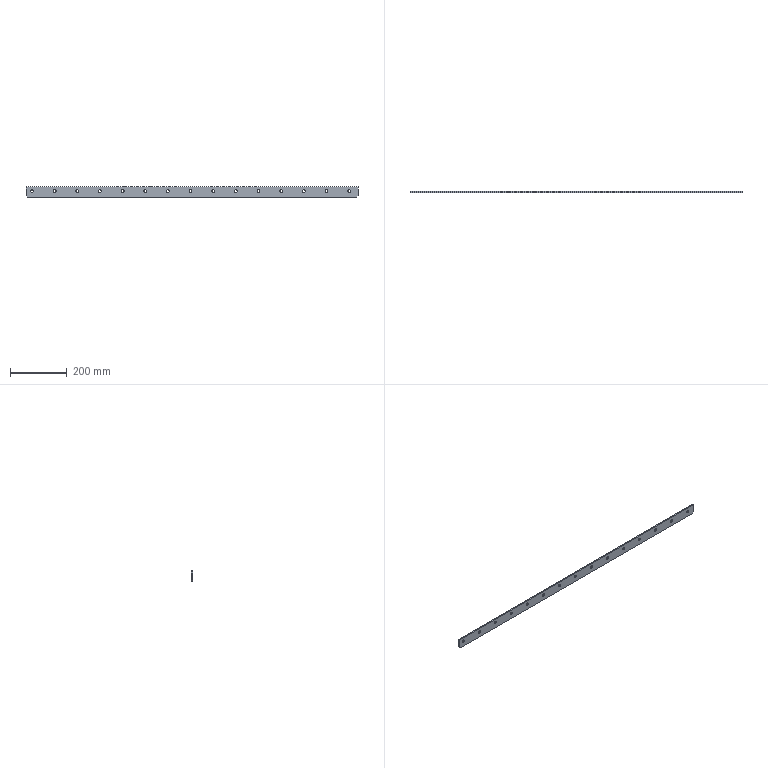Part | SolidWorks | features Chamfer 1, Extrusion 1, HoleWzd 1, LPattern 1 | 1 solid | 38 faces | box 1172 x 4 x 36 mm | volume 163956 mm3 | cylinder 30 | plane 8 | commonest cylinder face diameters 10 x30
STEP:
#1=CARTESIAN_POINT('',(-31.,0.,16.));
#2=VERTEX_POINT('',#1);
#3=CARTESIAN_POINT('',(-31.,0.,26.));
#4=VERTEX_POINT('',#3);
#5=CARTESIAN_POINT('',(-31.,0.,21.));
#6=DIRECTION('',(0.,1.,0.));
#7=DIRECTION('',(0.,0.,1.));
#8=AXIS2_PLACEMENT_3D('',#5,#6,#7);
#9=CIRCLE('',#8,5.);
#10=EDGE_CURVE('',#2,#4,#9,.T.);
#11=ORIENTED_EDGE('',*,*,#10,.F.);
#12=CARTESIAN_POINT('',(-31.,4.,16.));
#13=VERTEX_POINT('',#12);
#14=CARTESIAN_POINT('',(-31.,4.,16.));
#15=DIRECTION('',(0.,1.,0.));
#16=VECTOR('',#15,1000.);
#17=LINE('',#14,#16);
#18=EDGE_CURVE('',#2,#13,#17,.T.);
#19=ORIENTED_EDGE('',*,*,#18,.T.);
#20=CARTESIAN_POINT('',(-31.,4.,26.));
#21=VERTEX_POINT('',#20);
#22=CARTESIAN_POINT('',(-31.,4.,21.));
#23=DIRECTION('',(0.,1.,0.));
#24=DIRECTION('',(0.,0.,1.));
#25=AXIS2_PLACEMENT_3D('',#22,#23,#24);
#26=CIRCLE('',#25,5.);
#27=EDGE_CURVE('',#13,#21,#26,.T.);
#28=ORIENTED_EDGE('',*,*,#27,.T.);
#29=CARTESIAN_POINT('',(-31.,4.,26.));
#30=DIRECTION('',(0.,1.,0.));
#31=VECTOR('',#30,1000.);
#32=LINE('',#29,#31);
#33=EDGE_CURVE('',#4,#21,#32,.T.);
#34=ORIENTED_EDGE('',*,*,#33,.F.);
#35=EDGE_LOOP('',(#11,#19,#28,#34));
#36=FACE_OUTER_BOUND('',#35,.T.);
#37=CARTESIAN_POINT('',(-31.,4.,21.));
#38=DIRECTION('',(0.,1.,0.));
#39=DIRECTION('',(0.,0.,1.));
#40=AXIS2_PLACEMENT_3D('',#37,#38,#39);
#41=CYLINDRICAL_SURFACE('',#40,5.);
#42=ADVANCED_FACE('',(#36),#41,.F.);
#43=CARTESIAN_POINT('',(-111.,0.,16.));
#44=VERTEX_POINT('',#43);
#45=CARTESIAN_POINT('',(-111.,0.,26.));
#46=VERTEX_POINT('',#45);
#47=CARTESIAN_POINT('',(-111.,0.,21.));
#48=DIRECTION('',(0.,1.,0.));
#49=DIRECTION('',(0.,0.,1.));
#50=AXIS2_PLACEMENT_3D('',#47,#48,#49);
#51=CIRCLE('',#50,5.);
#52=EDGE_CURVE('',#44,#46,#51,.T.);
#53=ORIENTED_EDGE('',*,*,#52,.F.);
#54=CARTESIAN_POINT('',(-111.,4.,16.));
#55=VERTEX_POINT('',#54);
#56=CARTESIAN_POINT('',(-111.,4.,16.));
#57=DIRECTION('',(0.,1.,0.));
#58=VECTOR('',#57,1000.);
#59=LINE('',#56,#58);
#60=EDGE_CURVE('',#44,#55,#59,.T.);
#61=ORIENTED_EDGE('',*,*,#60,.T.);
#62=CARTESIAN_POINT('',(-111.,4.,26.));
#63=VERTEX_POINT('',#62);
#64=CARTESIAN_POINT('',(-111.,4.,21.));
#65=DIRECTION('',(0.,1.,0.));
#66=DIRECTION('',(0.,0.,1.));
#67=AXIS2_PLACEMENT_3D('',#64,#65,#66);
#68=CIRCLE('',#67,5.);
#69=EDGE_CURVE('',#55,#63,#68,.T.);
#70=ORIENTED_EDGE('',*,*,#69,.T.);
#71=CARTESIAN_POINT('',(-111.,4.,26.));
#72=DIRECTION('',(0.,1.,0.));
#73=VECTOR('',#72,1000.);
#74=LINE('',#71,#73);
#75=EDGE_CURVE('',#46,#63,#74,.T.);
#76=ORIENTED_EDGE('',*,*,#75,.F.);
#77=EDGE_LOOP('',(#53,#61,#70,#76));
#78=FACE_OUTER_BOUND('',#77,.T.);
#79=CARTESIAN_POINT('',(-111.,4.,21.));
#80=DIRECTION('',(0.,1.,0.));
#81=DIRECTION('',(0.,0.,1.));
#82=AXIS2_PLACEMENT_3D('',#79,#80,#81);
#83=CYLINDRICAL_SURFACE('',#82,5.);
#84=ADVANCED_FACE('',(#78),#83,.F.);
#85=CARTESIAN_POINT('',(-191.,0.,16.));
#86=VERTEX_POINT('',#85);
#87=CARTESIAN_POINT('',(-191.,0.,26.));
#88=VERTEX_POINT('',#87);
#89=CARTESIAN_POINT('',(-191.,0.,21.));
#90=DIRECTION('',(0.,1.,0.));
#91=DIRECTION('',(0.,0.,1.));
#92=AXIS2_PLACEMENT_3D('',#89,#90,#91);
#93=CIRCLE('',#92,5.);
#94=EDGE_CURVE('',#86,#88,#93,.T.);
#95=ORIENTED_EDGE('',*,*,#94,.F.);
#96=CARTESIAN_POINT('',(-191.,4.,16.));
#97=VERTEX_POINT('',#96);
#98=CARTESIAN_POINT('',(-191.,4.,16.));
#99=DIRECTION('',(0.,1.,0.));
#100=VECTOR('',#99,1000.);
#101=LINE('',#98,#100);
#102=EDGE_CURVE('',#86,#97,#101,.T.);
#103=ORIENTED_EDGE('',*,*,#102,.T.);
#104=CARTESIAN_POINT('',(-191.,4.,26.));
#105=VERTEX_POINT('',#104);
#106=CARTESIAN_POINT('',(-191.,4.,21.));
#107=DIRECTION('',(0.,1.,0.));
#108=DIRECTION('',(0.,0.,1.));
#109=AXIS2_PLACEMENT_3D('',#106,#107,#108);
#110=CIRCLE('',#109,5.);
#111=EDGE_CURVE('',#97,#105,#110,.T.);
#112=ORIENTED_EDGE('',*,*,#111,.T.);
#113=CARTESIAN_POINT('',(-191.,4.,26.));
#114=DIRECTION('',(0.,1.,0.));
#115=VECTOR('',#114,1000.);
#116=LINE('',#113,#115);
#117=EDGE_CURVE('',#88,#105,#116,.T.);
#118=ORIENTED_EDGE('',*,*,#117,.F.);
#119=EDGE_LOOP('',(#95,#103,#112,#118));
#120=FACE_OUTER_BOUND('',#119,.T.);
#121=CARTESIAN_POINT('',(-191.,4.,21.));
#122=DIRECTION('',(0.,1.,0.));
#123=DIRECTION('',(0.,0.,1.));
#124=AXIS2_PLACEMENT_3D('',#121,#122,#123);
#125=CYLINDRICAL_SURFACE('',#124,5.);
#126=ADVANCED_FACE('',(#120),#125,.F.);
#127=CARTESIAN_POINT('',(-271.,0.,16.));
#128=VERTEX_POINT('',#127);
#129=CARTESIAN_POINT('',(-271.,0.,26.));
#130=VERTEX_POINT('',#129);
#131=CARTESIAN_POINT('',(-271.,0.,21.));
#132=DIRECTION('',(0.,1.,0.));
#133=DIRECTION('',(0.,0.,1.));
#134=AXIS2_PLACEMENT_3D('',#131,#132,#133);
#135=CIRCLE('',#134,5.);
#136=EDGE_CURVE('',#128,#130,#135,.T.);
#137=ORIENTED_EDGE('',*,*,#136,.F.);
#138=CARTESIAN_POINT('',(-271.,4.,16.));
#139=VERTEX_POINT('',#138);
#140=CARTESIAN_POINT('',(-271.,4.,16.));
#141=DIRECTION('',(0.,1.,0.));
#142=VECTOR('',#141,1000.);
#143=LINE('',#140,#142);
#144=EDGE_CURVE('',#128,#139,#143,.T.);
#145=ORIENTED_EDGE('',*,*,#144,.T.);
#146=CARTESIAN_POINT('',(-271.,4.,26.));
#147=VERTEX_POINT('',#146);
#148=CARTESIAN_POINT('',(-271.,4.,21.));
#149=DIRECTION('',(0.,1.,0.));
#150=DIRECTION('',(0.,0.,1.));
#151=AXIS2_PLACEMENT_3D('',#148,#149,#150);
#152=CIRCLE('',#151,5.);
#153=EDGE_CURVE('',#139,#147,#152,.T.);
#154=ORIENTED_EDGE('',*,*,#153,.T.);
#155=CARTESIAN_POINT('',(-271.,4.,26.));
#156=DIRECTION('',(0.,1.,0.));
#157=VECTOR('',#156,1000.);
#158=LINE('',#155,#157);
#159=EDGE_CURVE('',#130,#147,#158,.T.);
#160=ORIENTED_EDGE('',*,*,#159,.F.);
#161=EDGE_LOOP('',(#137,#145,#154,#160));
#162=FACE_OUTER_BOUND('',#161,.T.);
#163=CARTESIAN_POINT('',(-271.,4.,21.));
#164=DIRECTION('',(0.,1.,0.));
#165=DIRECTION('',(0.,0.,1.));
#166=AXIS2_PLACEMENT_3D('',#163,#164,#165);
#167=CYLINDRICAL_SURFACE('',#166,5.);
#168=ADVANCED_FACE('',(#162),#167,.F.);
#169=CARTESIAN_POINT('',(-351.,0.,16.));
#170=VERTEX_POINT('',#169);
#171=CARTESIAN_POINT('',(-351.,0.,26.));
#172=VERTEX_POINT('',#171);
#173=CARTESIAN_POINT('',(-351.,0.,21.));
#174=DIRECTION('',(0.,1.,0.));
#175=DIRECTION('',(0.,0.,1.));
#176=AXIS2_PLACEMENT_3D('',#173,#174,#175);
#177=CIRCLE('',#176,5.);
#178=EDGE_CURVE('',#170,#172,#177,.T.);
#179=ORIENTED_EDGE('',*,*,#178,.F.);
#180=CARTESIAN_POINT('',(-351.,4.,16.));
#181=VERTEX_POINT('',#180);
#182=CARTESIAN_POINT('',(-351.,4.,16.));
#183=DIRECTION('',(0.,1.,0.));
#184=VECTOR('',#183,1000.);
#185=LINE('',#182,#184);
#186=EDGE_CURVE('',#170,#181,#185,.T.);
#187=ORIENTED_EDGE('',*,*,#186,.T.);
#188=CARTESIAN_POINT('',(-351.,4.,26.));
#189=VERTEX_POINT('',#188);
#190=CARTESIAN_POINT('',(-351.,4.,21.));
#191=DIRECTION('',(0.,1.,0.));
#192=DIRECTION('',(0.,0.,1.));
#193=AXIS2_PLACEMENT_3D('',#190,#191,#192);
#194=CIRCLE('',#193,5.);
#195=EDGE_CURVE('',#181,#189,#194,.T.);
#196=ORIENTED_EDGE('',*,*,#195,.T.);
#197=CARTESIAN_POINT('',(-351.,4.,26.));
#198=DIRECTION('',(0.,1.,0.));
#199=VECTOR('',#198,1000.);
#200=LINE('',#197,#199);
#201=EDGE_CURVE('',#172,#189,#200,.T.);
#202=ORIENTED_EDGE('',*,*,#201,.F.);
#203=EDGE_LOOP('',(#179,#187,#196,#202));
#204=FACE_OUTER_BOUND('',#203,.T.);
#205=CARTESIAN_POINT('',(-351.,4.,21.));
#206=DIRECTION('',(0.,1.,0.));
#207=DIRECTION('',(0.,0.,1.));
#208=AXIS2_PLACEMENT_3D('',#205,#206,#207);
#209=CYLINDRICAL_SURFACE('',#208,5.);
#210=ADVANCED_FACE('',(#204),#209,.F.);
#211=CARTESIAN_POINT('',(-431.,0.,16.));
#212=VERTEX_POINT('',#211);
#213=CARTESIAN_POINT('',(-431.,0.,26.));
#214=VERTEX_POINT('',#213);
#215=CARTESIAN_POINT('',(-431.,0.,21.));
#216=DIRECTION('',(0.,1.,0.));
#217=DIRECTION('',(0.,0.,1.));
#218=AXIS2_PLACEMENT_3D('',#215,#216,#217);
#219=CIRCLE('',#218,5.);
#220=EDGE_CURVE('',#212,#214,#219,.T.);
#221=ORIENTED_EDGE('',*,*,#220,.F.);
#222=CARTESIAN_POINT('',(-431.,4.,16.));
#223=VERTEX_POINT('',#222);
#224=CARTESIAN_POINT('',(-431.,4.,16.));
#225=DIRECTION('',(0.,1.,0.));
#226=VECTOR('',#225,1000.);
#227=LINE('',#224,#226);
#228=EDGE_CURVE('',#212,#223,#227,.T.);
#229=ORIENTED_EDGE('',*,*,#228,.T.);
#230=CARTESIAN_POINT('',(-431.,4.,26.));
#231=VERTEX_POINT('',#230);
#232=CARTESIAN_POINT('',(-431.,4.,21.));
#233=DIRECTION('',(0.,1.,0.));
#234=DIRECTION('',(0.,0.,1.));
#235=AXIS2_PLACEMENT_3D('',#232,#233,#234);
#236=CIRCLE('',#235,5.);
#237=EDGE_CURVE('',#223,#231,#236,.T.);
#238=ORIENTED_EDGE('',*,*,#237,.T.);
#239=CARTESIAN_POINT('',(-431.,4.,26.));
#240=DIRECTION('',(0.,1.,0.));
#241=VECTOR('',#240,1000.);
#242=LINE('',#239,#241);
#243=EDGE_CURVE('',#214,#231,#242,.T.);
#244=ORIENTED_EDGE('',*,*,#243,.F.);
#245=EDGE_LOOP('',(#221,#229,#238,#244));
#246=FACE_OUTER_BOUND('',#245,.T.);
#247=CARTESIAN_POINT('',(-431.,4.,21.));
#248=DIRECTION('',(0.,1.,0.));
#249=DIRECTION('',(0.,0.,1.));
#250=AXIS2_PLACEMENT_3D('',#247,#248,#249);
#251=CYLINDRICAL_SURFACE('',#250,5.);
#252=ADVANCED_FACE('',(#246),#251,.F.);
#253=CARTESIAN_POINT('',(-511.,0.,16.));
#254=VERTEX_POINT('',#253);
#255=CARTESIAN_POINT('',(-511.,0.,26.));
#256=VERTEX_POINT('',#255);
#257=CARTESIAN_POINT('',(-511.,0.,21.));
#258=DIRECTION('',(0.,1.,0.));
#259=DIRECTION('',(0.,0.,1.));
#260=AXIS2_PLACEMENT_3D('',#257,#258,#259);
#261=CIRCLE('',#260,5.);
#262=EDGE_CURVE('',#254,#256,#261,.T.);
#263=ORIENTED_EDGE('',*,*,#262,.F.);
#264=CARTESIAN_POINT('',(-511.,4.,16.));
#265=VERTEX_POINT('',#264);
#266=CARTESIAN_POINT('',(-511.,4.,16.));
#267=DIRECTION('',(0.,1.,0.));
#268=VECTOR('',#267,1000.);
#269=LINE('',#266,#268);
#270=EDGE_CURVE('',#254,#265,#269,.T.);
#271=ORIENTED_EDGE('',*,*,#270,.T.);
#272=CARTESIAN_POINT('',(-511.,4.,26.));
#273=VERTEX_POINT('',#272);
#274=CARTESIAN_POINT('',(-511.,4.,21.));
#275=DIRECTION('',(0.,1.,0.));
#276=DIRECTION('',(0.,0.,1.));
#277=AXIS2_PLACEMENT_3D('',#274,#275,#276);
#278=CIRCLE('',#277,5.);
#279=EDGE_CURVE('',#265,#273,#278,.T.);
#280=ORIENTED_EDGE('',*,*,#279,.T.);
#281=CARTESIAN_POINT('',(-511.,4.,26.));
#282=DIRECTION('',(0.,1.,0.));
#283=VECTOR('',#282,1000.);
#284=LINE('',#281,#283);
#285=EDGE_CURVE('',#256,#273,#284,.T.);
#286=ORIENTED_EDGE('',*,*,#285,.F.);
#287=EDGE_LOOP('',(#263,#271,#280,#286));
#288=FACE_OUTER_BOUND('',#287,.T.);
#289=CARTESIAN_POINT('',(-511.,4.,21.));
#290=DIRECTION('',(0.,1.,0.));
#291=DIRECTION('',(0.,0.,1.));
#292=AXIS2_PLACEMENT_3D('',#289,#290,#291);
#293=CYLINDRICAL_SURFACE('',#292,5.);
#294=ADVANCED_FACE('',(#288),#293,.F.);
#295=CARTESIAN_POINT('',(-591.,0.,16.));
#296=VERTEX_POINT('',#295);
#297=CARTESIAN_POINT('',(-591.,0.,26.));
#298=VERTEX_POINT('',#297);
#299=CARTESIAN_POINT('',(-591.,0.,21.));
#300=DIRECTION('',(0.,1.,0.));
#301=DIRECTION('',(0.,0.,1.));
#302=AXIS2_PLACEMENT_3D('',#299,#300,#301);
#303=CIRCLE('',#302,5.);
#304=EDGE_CURVE('',#296,#298,#303,.T.);
#305=ORIENTED_EDGE('',*,*,#304,.F.);
#306=CARTESIAN_POINT('',(-591.,4.,16.));
#307=VERTEX_POINT('',#306);
#308=CARTESIAN_POINT('',(-591.,4.,16.));
#309=DIRECTION('',(0.,1.,0.));
#310=VECTOR('',#309,1000.);
#311=LINE('',#308,#310);
#312=EDGE_CURVE('',#296,#307,#311,.T.);
#313=ORIENTED_EDGE('',*,*,#312,.T.);
#314=CARTESIAN_POINT('',(-591.,4.,26.));
#315=VERTEX_POINT('',#314);
#316=CARTESIAN_POINT('',(-591.,4.,21.));
#317=DIRECTION('',(0.,1.,0.));
#318=DIRECTION('',(0.,0.,1.));
#319=AXIS2_PLACEMENT_3D('',#316,#317,#318);
#320=CIRCLE('',#319,5.);
#321=EDGE_CURVE('',#307,#315,#320,.T.);
#322=ORIENTED_EDGE('',*,*,#321,.T.);
#323=CARTESIAN_POINT('',(-591.,4.,26.));
#324=DIRECTION('',(0.,1.,0.));
#325=VECTOR('',#324,1000.);
#326=LINE('',#323,#325);
#327=EDGE_CURVE('',#298,#315,#326,.T.);
#328=ORIENTED_EDGE('',*,*,#327,.F.);
#329=EDGE_LOOP('',(#305,#313,#322,#328));
#330=FACE_OUTER_BOUND('',#329,.T.);
#331=CARTESIAN_POINT('',(-591.,4.,21.));
#332=DIRECTION('',(0.,1.,0.));
#333=DIRECTION('',(0.,0.,1.));
#334=AXIS2_PLACEMENT_3D('',#331,#332,#333);
#335=CYLINDRICAL_SURFACE('',#334,5.);
#336=ADVANCED_FACE('',(#330),#335,.F.);
#337=CARTESIAN_POINT('',(-671.,0.,16.));
#338=VERTEX_POINT('',#337);
#339=CARTESIAN_POINT('',(-671.,0.,26.));
#340=VERTEX_POINT('',#339);
#341=CARTESIAN_POINT('',(-671.,0.,21.));
#342=DIRECTION('',(0.,1.,0.));
#343=DIRECTION('',(0.,0.,1.));
#344=AXIS2_PLACEMENT_3D('',#341,#342,#343);
#345=CIRCLE('',#344,5.);
#346=EDGE_CURVE('',#338,#340,#345,.T.);
#347=ORIENTED_EDGE('',*,*,#346,.F.);
#348=CARTESIAN_POINT('',(-671.,4.,16.));
#349=VERTEX_POINT('',#348);
#350=CARTESIAN_POINT('',(-671.,4.,16.));
#351=DIRECTION('',(0.,1.,0.));
#352=VECTOR('',#351,1000.);
#353=LINE('',#350,#352);
#354=EDGE_CURVE('',#338,#349,#353,.T.);
#355=ORIENTED_EDGE('',*,*,#354,.T.);
#356=CARTESIAN_POINT('',(-671.,4.,26.));
#357=VERTEX_POINT('',#356);
#358=CARTESIAN_POINT('',(-671.,4.,21.));
#359=DIRECTION('',(0.,1.,0.));
#360=DIRECTION('',(0.,0.,1.));
#361=AXIS2_PLACEMENT_3D('',#358,#359,#360);
#362=CIRCLE('',#361,5.);
#363=EDGE_CURVE('',#349,#357,#362,.T.);
#364=ORIENTED_EDGE('',*,*,#363,.T.);
#365=CARTESIAN_POINT('',(-671.,4.,26.));
#366=DIRECTION('',(0.,1.,0.));
#367=VECTOR('',#366,1000.);
#368=LINE('',#365,#367);
#369=EDGE_CURVE('',#340,#357,#368,.T.);
#370=ORIENTED_EDGE('',*,*,#369,.F.);
#371=EDGE_LOOP('',(#347,#355,#364,#370));
#372=FACE_OUTER_BOUND('',#371,.T.);
#373=CARTESIAN_POINT('',(-671.,4.,21.));
#374=DIRECTION('',(0.,1.,0.));
#375=DIRECTION('',(0.,0.,1.));
#376=AXIS2_PLACEMENT_3D('',#373,#374,#375);
#377=CYLINDRICAL_SURFACE('',#376,5.);
#378=ADVANCED_FACE('',(#372),#377,.F.);
#379=CARTESIAN_POINT('',(-751.,0.,16.));
#380=VERTEX_POINT('',#379);
#381=CARTESIAN_POINT('',(-751.,0.,26.));
#382=VERTEX_POINT('',#381);
#383=CARTESIAN_POINT('',(-751.,0.,21.));
#384=DIRECTION('',(0.,1.,0.));
#385=DIRECTION('',(0.,0.,1.));
#386=AXIS2_PLACEMENT_3D('',#383,#384,#385);
#387=CIRCLE('',#386,5.);
#388=EDGE_CURVE('',#380,#382,#387,.T.);
#389=ORIENTED_EDGE('',*,*,#388,.F.);
#390=CARTESIAN_POINT('',(-751.,4.,16.));
#391=VERTEX_POINT('',#390);
#392=CARTESIAN_POINT('',(-751.,4.,16.));
#393=DIRECTION('',(0.,1.,0.));
#394=VECTOR('',#393,1000.);
#395=LINE('',#392,#394);
#396=EDGE_CURVE('',#380,#391,#395,.T.);
#397=ORIENTED_EDGE('',*,*,#396,.T.);
#398=CARTESIAN_POINT('',(-751.,4.,26.));
#399=VERTEX_POINT('',#398);
#400=CARTESIAN_POINT('',(-751.,4.,21.));
#401=DIRECTION('',(0.,1.,0.));
#402=DIRECTION('',(0.,0.,1.));
#403=AXIS2_PLACEMENT_3D('',#400,#401,#402);
#404=CIRCLE('',#403,5.);
#405=EDGE_CURVE('',#391,#399,#404,.T.);
#406=ORIENTED_EDGE('',*,*,#405,.T.);
#407=CARTESIAN_POINT('',(-751.,4.,26.));
#408=DIRECTION('',(0.,1.,0.));
#409=VECTOR('',#408,1000.);
#410=LINE('',#407,#409);
#411=EDGE_CURVE('',#382,#399,#410,.T.);
#412=ORIENTED_EDGE('',*,*,#411,.F.);
#413=EDGE_LOOP('',(#389,#397,#406,#412));
#414=FACE_OUTER_BOUND('',#413,.T.);
#415=CARTESIAN_POINT('',(-751.,4.,21.));
#416=DIRECTION('',(0.,1.,0.));
#417=DIRECTION('',(0.,0.,1.));
#418=AXIS2_PLACEMENT_3D('',#415,#416,#417);
#419=CYLINDRICAL_SURFACE('',#418,5.);
#420=ADVANCED_FACE('',(#414),#419,.F.);
#421=CARTESIAN_POINT('',(-831.,0.,16.));
#422=VERTEX_POINT('',#421);
#423=CARTESIAN_POINT('',(-831.,0.,26.));
#424=VERTEX_POINT('',#423);
#425=CARTESIAN_POINT('',(-831.,0.,21.));
#426=DIRECTION('',(0.,1.,0.));
#427=DIRECTION('',(0.,0.,1.));
#428=AXIS2_PLACEMENT_3D('',#425,#426,#427);
#429=CIRCLE('',#428,5.);
#430=EDGE_CURVE('',#422,#424,#429,.T.);
#431=ORIENTED_EDGE('',*,*,#430,.F.);
#432=CARTESIAN_POINT('',(-831.,4.,16.));
#433=VERTEX_POINT('',#432);
#434=CARTESIAN_POINT('',(-831.,4.,16.));
#435=DIRECTION('',(0.,1.,0.));
#436=VECTOR('',#435,1000.);
#437=LINE('',#434,#436);
#438=EDGE_CURVE('',#422,#433,#437,.T.);
#439=ORIENTED_EDGE('',*,*,#438,.T.);
#440=CARTESIAN_POINT('',(-831.,4.,26.));
#441=VERTEX_POINT('',#440);
#442=CARTESIAN_POINT('',(-831.,4.,21.));
#443=DIRECTION('',(0.,1.,0.));
#444=DIRECTION('',(0.,0.,1.));
#445=AXIS2_PLACEMENT_3D('',#442,#443,#444);
#446=CIRCLE('',#445,5.);
#447=EDGE_CURVE('',#433,#441,#446,.T.);
#448=ORIENTED_EDGE('',*,*,#447,.T.);
#449=CARTESIAN_POINT('',(-831.,4.,26.));
#450=DIRECTION('',(0.,1.,0.));
#451=VECTOR('',#450,1000.);
#452=LINE('',#449,#451);
#453=EDGE_CURVE('',#424,#441,#452,.T.);
#454=ORIENTED_EDGE('',*,*,#453,.F.);
#455=EDGE_LOOP('',(#431,#439,#448,#454));
#456=FACE_OUTER_BOUND('',#455,.T.);
#457=CARTESIAN_POINT('',(-831.,4.,21.));
#458=DIRECTION('',(0.,1.,0.));
#459=DIRECTION('',(0.,0.,1.));
#460=AXIS2_PLACEMENT_3D('',#457,#458,#459);
#461=CYLINDRICAL_SURFACE('',#460,5.);
#462=ADVANCED_FACE('',(#456),#461,.F.);
#463=CARTESIAN_POINT('',(-911.,0.,16.));
#464=VERTEX_POINT('',#463);
#465=CARTESIAN_POINT('',(-911.,0.,26.));
#466=VERTEX_POINT('',#465);
#467=CARTESIAN_POINT('',(-911.,0.,21.));
#468=DIRECTION('',(0.,1.,0.));
#469=DIRECTION('',(0.,0.,1.));
#470=AXIS2_PLACEMENT_3D('',#467,#468,#469);
#471=CIRCLE('',#470,5.);
#472=EDGE_CURVE('',#464,#466,#471,.T.);
#473=ORIENTED_EDGE('',*,*,#472,.F.);
#474=CARTESIAN_POINT('',(-911.,4.,16.));
#475=VERTEX_POINT('',#474);
#476=CARTESIAN_POINT('',(-911.,4.,16.));
#477=DIRECTION('',(0.,1.,0.));
#478=VECTOR('',#477,1000.);
#479=LINE('',#476,#478);
#480=EDGE_CURVE('',#464,#475,#479,.T.);
#481=ORIENTED_EDGE('',*,*,#480,.T.);
#482=CARTESIAN_POINT('',(-911.,4.,26.));
#483=VERTEX_POINT('',#482);
#484=CARTESIAN_POINT('',(-911.,4.,21.));
#485=DIRECTION('',(0.,1.,0.));
#486=DIRECTION('',(0.,0.,1.));
#487=AXIS2_PLACEMENT_3D('',#484,#485,#486);
#488=CIRCLE('',#487,5.);
#489=EDGE_CURVE('',#475,#483,#488,.T.);
#490=ORIENTED_EDGE('',*,*,#489,.T.);
#491=CARTESIAN_POINT('',(-911.,4.,26.));
#492=DIRECTION('',(0.,1.,0.));
#493=VECTOR('',#492,1000.);
#494=LINE('',#491,#493);
#495=EDGE_CURVE('',#466,#483,#494,.T.);
#496=ORIENTED_EDGE('',*,*,#495,.F.);
#497=EDGE_LOOP('',(#473,#481,#490,#496));
#498=FACE_OUTER_BOUND('',#497,.T.);
#499=CARTESIAN_POINT('',(-911.,4.,21.));
#500=DIRECTION('',(0.,1.,0.));
#501=DIRECTION('',(0.,0.,1.));
#502=AXIS2_PLACEMENT_3D('',#499,#500,#501);
#503=CYLINDRICAL_SURFACE('',#502,5.);
#504=ADVANCED_FACE('',(#498),#503,.F.);
#505=CARTESIAN_POINT('',(-991.,0.,16.));
#506=VERTEX_POINT('',#505);
#507=CARTESIAN_POINT('',(-991.,0.,26.));
#508=VERTEX_POINT('',#507);
#509=CARTESIAN_POINT('',(-991.,0.,21.));
#510=DIRECTION('',(0.,1.,0.));
#511=DIRECTION('',(0.,0.,1.));
#512=AXIS2_PLACEMENT_3D('',#509,#510,#511);
#513=CIRCLE('',#512,5.);
#514=EDGE_CURVE('',#506,#508,#513,.T.);
#515=ORIENTED_EDGE('',*,*,#514,.F.);
#516=CARTESIAN_POINT('',(-991.,4.,16.));
#517=VERTEX_POINT('',#516);
#518=CARTESIAN_POINT('',(-991.,4.,16.));
#519=DIRECTION('',(0.,1.,0.));
#520=VECTOR('',#519,1000.);
#521=LINE('',#518,#520);
#522=EDGE_CURVE('',#506,#517,#521,.T.);
#523=ORIENTED_EDGE('',*,*,#522,.T.);
#524=CARTESIAN_POINT('',(-991.,4.,26.));
#525=VERTEX_POINT('',#524);
#526=CARTESIAN_POINT('',(-991.,4.,21.));
#527=DIRECTION('',(0.,1.,0.));
#528=DIRECTION('',(0.,0.,1.));
#529=AXIS2_PLACEMENT_3D('',#526,#527,#528);
#530=CIRCLE('',#529,5.);
#531=EDGE_CURVE('',#517,#525,#530,.T.);
#532=ORIENTED_EDGE('',*,*,#531,.T.);
#533=CARTESIAN_POINT('',(-991.,4.,26.));
#534=DIRECTION('',(0.,1.,0.));
#535=VECTOR('',#534,1000.);
#536=LINE('',#533,#535);
#537=EDGE_CURVE('',#508,#525,#536,.T.);
#538=ORIENTED_EDGE('',*,*,#537,.F.);
#539=EDGE_LOOP('',(#515,#523,#532,#538));
#540=FACE_OUTER_BOUND('',#539,.T.);
#541=CARTESIAN_POINT('',(-991.,4.,21.));
#542=DIRECTION('',(0.,1.,0.));
#543=DIRECTION('',(0.,0.,1.));
#544=AXIS2_PLACEMENT_3D('',#541,#542,#543);
#545=CYLINDRICAL_SURFACE('',#544,5.);
#546=ADVANCED_FACE('',(#540),#545,.F.);
#547=CARTESIAN_POINT('',(-1071.,0.,16.));
#548=VERTEX_POINT('',#547);
#549=CARTESIAN_POINT('',(-1071.,0.,26.));
#550=VERTEX_POINT('',#549);
#551=CARTESIAN_POINT('',(-1071.,0.,21.));
#552=DIRECTION('',(0.,1.,0.));
#553=DIRECTION('',(0.,0.,1.));
#554=AXIS2_PLACEMENT_3D('',#551,#552,#553);
#555=CIRCLE('',#554,5.);
#556=EDGE_CURVE('',#548,#550,#555,.T.);
#557=ORIENTED_EDGE('',*,*,#556,.F.);
#558=CARTESIAN_POINT('',(-1071.,4.,16.));
#559=VERTEX_POINT('',#558);
#560=CARTESIAN_POINT('',(-1071.,4.,16.));
#561=DIRECTION('',(0.,1.,0.));
#562=VECTOR('',#561,1000.);
#563=LINE('',#560,#562);
#564=EDGE_CURVE('',#548,#559,#563,.T.);
#565=ORIENTED_EDGE('',*,*,#564,.T.);
#566=CARTESIAN_POINT('',(-1071.,4.,26.));
#567=VERTEX_POINT('',#566);
#568=CARTESIAN_POINT('',(-1071.,4.,21.));
#569=DIRECTION('',(0.,1.,0.));
#570=DIRECTION('',(0.,0.,1.));
#571=AXIS2_PLACEMENT_3D('',#568,#569,#570);
#572=CIRCLE('',#571,5.);
#573=EDGE_CURVE('',#559,#567,#572,.T.);
#574=ORIENTED_EDGE('',*,*,#573,.T.);
#575=CARTESIAN_POINT('',(-1071.,4.,26.));
#576=DIRECTION('',(0.,1.,0.));
#577=VECTOR('',#576,1000.);
#578=LINE('',#575,#577);
#579=EDGE_CURVE('',#550,#567,#578,.T.);
#580=ORIENTED_EDGE('',*,*,#579,.F.);
#581=EDGE_LOOP('',(#557,#565,#574,#580));
#582=FACE_OUTER_BOUND('',#581,.T.);
#583=CARTESIAN_POINT('',(-1071.,4.,21.));
#584=DIRECTION('',(0.,1.,0.));
#585=DIRECTION('',(0.,0.,1.));
#586=AXIS2_PLACEMENT_3D('',#583,#584,#585);
#587=CYLINDRICAL_SURFACE('',#586,5.);
#588=ADVANCED_FACE('',(#582),#587,.F.);
#589=CARTESIAN_POINT('',(-1151.,0.,16.));
#590=VERTEX_POINT('',#589);
#591=CARTESIAN_POINT('',(-1151.,0.,26.));
#592=VERTEX_POINT('',#591);
#593=CARTESIAN_POINT('',(-1151.,0.,21.));
#594=DIRECTION('',(0.,1.,0.));
#595=DIRECTION('',(0.,0.,1.));
#596=AXIS2_PLACEMENT_3D('',#593,#594,#595);
#597=CIRCLE('',#596,5.);
#598=EDGE_CURVE('',#590,#592,#597,.T.);
#599=ORIENTED_EDGE('',*,*,#598,.F.);
#600=CARTESIAN_POINT('',(-1151.,4.,16.));
#601=VERTEX_POINT('',#600);
#602=CARTESIAN_POINT('',(-1151.,4.,16.));
#603=DIRECTION('',(0.,1.,0.));
#604=VECTOR('',#603,1000.);
#605=LINE('',#602,#604);
#606=EDGE_CURVE('',#590,#601,#605,.T.);
#607=ORIENTED_EDGE('',*,*,#606,.T.);
#608=CARTESIAN_POINT('',(-1151.,4.,26.));
#609=VERTEX_POINT('',#608);
#610=CARTESIAN_POINT('',(-1151.,4.,21.));
#611=DIRECTION('',(0.,1.,0.));
#612=DIRECTION('',(0.,0.,1.));
#613=AXIS2_PLACEMENT_3D('',#610,#611,#612);
#614=CIRCLE('',#613,5.);
#615=EDGE_CURVE('',#601,#609,#614,.T.);
#616=ORIENTED_EDGE('',*,*,#615,.T.);
#617=CARTESIAN_POINT('',(-1151.,4.,26.));
#618=DIRECTION('',(0.,1.,0.));
#619=VECTOR('',#618,1000.);
#620=LINE('',#617,#619);
#621=EDGE_CURVE('',#592,#609,#620,.T.);
#622=ORIENTED_EDGE('',*,*,#621,.F.);
#623=EDGE_LOOP('',(#599,#607,#616,#622));
#624=FACE_OUTER_BOUND('',#623,.T.);
#625=CARTESIAN_POINT('',(-1151.,4.,21.));
#626=DIRECTION('',(0.,1.,0.));
#627=DIRECTION('',(0.,0.,1.));
#628=AXIS2_PLACEMENT_3D('',#625,#626,#627);
#629=CYLINDRICAL_SURFACE('',#628,5.);
#630=ADVANCED_FACE('',(#624),#629,.F.);
#631=CARTESIAN_POINT('',(-1172.,4.,5.));
#632=VERTEX_POINT('',#631);
#633=CARTESIAN_POINT('',(-1172.,4.,36.));
#634=VERTEX_POINT('',#633);
#635=CARTESIAN_POINT('',(-1172.,4.,0.));
#636=DIRECTION('',(0.,0.,1.));
#637=VECTOR('',#636,1000.);
#638=LINE('',#635,#637);
#639=EDGE_CURVE('',#632,#634,#638,.T.);
#640=ORIENTED_EDGE('',*,*,#639,.F.);
#641=CARTESIAN_POINT('',(-1172.,0.,5.));
#642=VERTEX_POINT('',#641);
#643=CARTESIAN_POINT('',(-1172.,4.,5.));
#644=DIRECTION('',(0.,-1.,0.));
#645=VECTOR('',#644,1000.);
#646=LINE('',#643,#645);
#647=EDGE_CURVE('',#632,#642,#646,.T.);
#648=ORIENTED_EDGE('',*,*,#647,.T.);
#649=CARTESIAN_POINT('',(-1172.,0.,36.));
#650=VERTEX_POINT('',#649);
#651=CARTESIAN_POINT('',(-1172.,0.,0.));
#652=DIRECTION('',(0.,0.,1.));
#653=VECTOR('',#652,1000.);
#654=LINE('',#651,#653);
#655=EDGE_CURVE('',#642,#650,#654,.T.);
#656=ORIENTED_EDGE('',*,*,#655,.T.);
#657=CARTESIAN_POINT('',(-1172.,4.,36.));
#658=DIRECTION('',(0.,-1.,0.));
#659=VECTOR('',#658,1000.);
#660=LINE('',#657,#659);
#661=EDGE_CURVE('',#634,#650,#660,.T.);
#662=ORIENTED_EDGE('',*,*,#661,.F.);
#663=EDGE_LOOP('',(#640,#648,#656,#662));
#664=FACE_OUTER_BOUND('',#663,.T.);
#665=CARTESIAN_POINT('',(-1172.,4.,0.));
#666=DIRECTION('',(1.,0.,0.));
#667=DIRECTION('',(0.,0.,-1.));
#668=AXIS2_PLACEMENT_3D('',#665,#666,#667);
#669=PLANE('',#668);
#670=ADVANCED_FACE('',(#664),#669,.F.);
#671=CARTESIAN_POINT('',(0.,0.,36.));
#672=VERTEX_POINT('',#671);
#673=CARTESIAN_POINT('',(-1172.,0.,36.));
#674=DIRECTION('',(1.,0.,0.));
#675=VECTOR('',#674,1000.);
#676=LINE('',#673,#675);
#677=EDGE_CURVE('',#650,#672,#676,.T.);
#678=ORIENTED_EDGE('',*,*,#677,.T.);
#679=CARTESIAN_POINT('',(0.,4.,36.));
#680=VERTEX_POINT('',#679);
#681=CARTESIAN_POINT('',(0.,4.,36.));
#682=DIRECTION('',(0.,-1.,0.));
#683=VECTOR('',#682,1000.);
#684=LINE('',#681,#683);
#685=EDGE_CURVE('',#680,#672,#684,.T.);
#686=ORIENTED_EDGE('',*,*,#685,.F.);
#687=CARTESIAN_POINT('',(-1172.,4.,36.));
#688=DIRECTION('',(1.,0.,0.));
#689=VECTOR('',#688,1000.);
#690=LINE('',#687,#689);
#691=EDGE_CURVE('',#634,#680,#690,.T.);
#692=ORIENTED_EDGE('',*,*,#691,.F.);
#693=ORIENTED_EDGE('',*,*,#661,.T.);
#694=EDGE_LOOP('',(#678,#686,#692,#693));
#695=FACE_OUTER_BOUND('',#694,.T.);
#696=CARTESIAN_POINT('',(-1172.,4.,36.));
#697=DIRECTION('',(0.,0.,-1.));
#698=DIRECTION('',(-1.,0.,0.));
#699=AXIS2_PLACEMENT_3D('',#696,#697,#698);
#700=PLANE('',#699);
#701=ADVANCED_FACE('',(#695),#700,.F.);
#702=CARTESIAN_POINT('',(0.,0.,5.));
#703=VERTEX_POINT('',#702);
#704=CARTESIAN_POINT('',(0.,0.,0.));
#705=DIRECTION('',(0.,0.,-1.));
#706=VECTOR('',#705,1000.);
#707=LINE('',#704,#706);
#708=EDGE_CURVE('',#672,#703,#707,.T.);
#709=ORIENTED_EDGE('',*,*,#708,.T.);
#710=CARTESIAN_POINT('',(0.,4.,5.));
#711=VERTEX_POINT('',#710);
#712=CARTESIAN_POINT('',(0.,4.,5.));
#713=DIRECTION('',(0.,1.,0.));
#714=VECTOR('',#713,1000.);
#715=LINE('',#712,#714);
#716=EDGE_CURVE('',#703,#711,#715,.T.);
#717=ORIENTED_EDGE('',*,*,#716,.T.);
#718=CARTESIAN_POINT('',(0.,4.,0.));
#719=DIRECTION('',(0.,0.,-1.));
#720=VECTOR('',#719,1000.);
#721=LINE('',#718,#720);
#722=EDGE_CURVE('',#680,#711,#721,.T.);
#723=ORIENTED_EDGE('',*,*,#722,.F.);
#724=ORIENTED_EDGE('',*,*,#685,.T.);
#725=EDGE_LOOP('',(#709,#717,#723,#724));
#726=FACE_OUTER_BOUND('',#725,.T.);
#727=CARTESIAN_POINT('',(0.,4.,0.));
#728=DIRECTION('',(-1.,0.,0.));
#729=DIRECTION('',(0.,0.,1.));
#730=AXIS2_PLACEMENT_3D('',#727,#728,#729);
#731=PLANE('',#730);
#732=ADVANCED_FACE('',(#726),#731,.F.);
#733=CARTESIAN_POINT('',(-5.,0.,0.));
#734=VERTEX_POINT('',#733);
#735=CARTESIAN_POINT('',(-1167.,0.,0.));
#736=VERTEX_POINT('',#735);
#737=CARTESIAN_POINT('',(-1172.,0.,0.));
#738=DIRECTION('',(-1.,0.,0.));
#739=VECTOR('',#738,1000.);
#740=LINE('',#737,#739);
#741=EDGE_CURVE('',#734,#736,#740,.T.);
#742=ORIENTED_EDGE('',*,*,#741,.T.);
#743=CARTESIAN_POINT('',(-1167.,4.,0.));
#744=VERTEX_POINT('',#743);
#745=CARTESIAN_POINT('',(-1167.,4.,0.));
#746=DIRECTION('',(0.,1.,0.));
#747=VECTOR('',#746,1000.);
#748=LINE('',#745,#747);
#749=EDGE_CURVE('',#736,#744,#748,.T.);
#750=ORIENTED_EDGE('',*,*,#749,.T.);
#751=CARTESIAN_POINT('',(-5.,4.,0.));
#752=VERTEX_POINT('',#751);
#753=CARTESIAN_POINT('',(-1172.,4.,0.));
#754=DIRECTION('',(-1.,0.,0.));
#755=VECTOR('',#754,1000.);
#756=LINE('',#753,#755);
#757=EDGE_CURVE('',#752,#744,#756,.T.);
#758=ORIENTED_EDGE('',*,*,#757,.F.);
#759=CARTESIAN_POINT('',(-5.,4.,0.));
#760=DIRECTION('',(0.,-1.,0.));
#761=VECTOR('',#760,1000.);
#762=LINE('',#759,#761);
#763=EDGE_CURVE('',#752,#734,#762,.T.);
#764=ORIENTED_EDGE('',*,*,#763,.T.);
#765=EDGE_LOOP('',(#742,#750,#758,#764));
#766=FACE_OUTER_BOUND('',#765,.T.);
#767=CARTESIAN_POINT('',(-1172.,4.,0.));
#768=DIRECTION('',(0.,0.,1.));
#769=DIRECTION('',(1.,0.,0.));
#770=AXIS2_PLACEMENT_3D('',#767,#768,#769);
#771=PLANE('',#770);
#772=ADVANCED_FACE('',(#766),#771,.F.);
#773=CARTESIAN_POINT('',(-1071.,4.,21.));
#774=DIRECTION('',(0.,1.,0.));
#775=DIRECTION('',(0.,0.,1.));
#776=AXIS2_PLACEMENT_3D('',#773,#774,#775);
#777=CIRCLE('',#776,5.);
#778=EDGE_CURVE('',#567,#559,#777,.T.);
#779=ORIENTED_EDGE('',*,*,#778,.F.);
#780=ORIENTED_EDGE('',*,*,#573,.F.);
#781=EDGE_LOOP('',(#779,#780));
#782=FACE_BOUND('',#781,.T.);
#783=CARTESIAN_POINT('',(-1151.,4.,21.));
#784=DIRECTION('',(0.,1.,0.));
#785=DIRECTION('',(0.,0.,1.));
#786=AXIS2_PLACEMENT_3D('',#783,#784,#785);
#787=CIRCLE('',#786,5.);
#788=EDGE_CURVE('',#609,#601,#787,.T.);
#789=ORIENTED_EDGE('',*,*,#788,.F.);
#790=ORIENTED_EDGE('',*,*,#615,.F.);
#791=EDGE_LOOP('',(#789,#790));
#792=FACE_BOUND('',#791,.T.);
#793=ORIENTED_EDGE('',*,*,#757,.T.);
#794=CARTESIAN_POINT('',(-1187.5,4.,20.5));
#795=DIRECTION('',(-0.7071,0.,0.7071));
#796=VECTOR('',#795,1000.);
#797=LINE('',#794,#796);
#798=EDGE_CURVE('',#744,#632,#797,.T.);
#799=ORIENTED_EDGE('',*,*,#798,.T.);
#800=ORIENTED_EDGE('',*,*,#639,.T.);
#801=ORIENTED_EDGE('',*,*,#691,.T.);
#802=ORIENTED_EDGE('',*,*,#722,.T.);
#803=CARTESIAN_POINT('',(-570.5,4.,-565.5));
#804=DIRECTION('',(-0.7071,0.,-0.7071));
#805=VECTOR('',#804,1000.);
#806=LINE('',#803,#805);
#807=EDGE_CURVE('',#711,#752,#806,.T.);
#808=ORIENTED_EDGE('',*,*,#807,.T.);
#809=EDGE_LOOP('',(#793,#799,#800,#801,#802,#808));
#810=FACE_OUTER_BOUND('',#809,.T.);
#811=CARTESIAN_POINT('',(-991.,4.,21.));
#812=DIRECTION('',(0.,1.,0.));
#813=DIRECTION('',(0.,0.,1.));
#814=AXIS2_PLACEMENT_3D('',#811,#812,#813);
#815=CIRCLE('',#814,5.);
#816=EDGE_CURVE('',#525,#517,#815,.T.);
#817=ORIENTED_EDGE('',*,*,#816,.F.);
#818=ORIENTED_EDGE('',*,*,#531,.F.);
#819=EDGE_LOOP('',(#817,#818));
#820=FACE_BOUND('',#819,.T.);
#821=CARTESIAN_POINT('',(-911.,4.,21.));
#822=DIRECTION('',(0.,1.,0.));
#823=DIRECTION('',(0.,0.,1.));
#824=AXIS2_PLACEMENT_3D('',#821,#822,#823);
#825=CIRCLE('',#824,5.);
#826=EDGE_CURVE('',#483,#475,#825,.T.);
#827=ORIENTED_EDGE('',*,*,#826,.F.);
#828=ORIENTED_EDGE('',*,*,#489,.F.);
#829=EDGE_LOOP('',(#827,#828));
#830=FACE_BOUND('',#829,.T.);
#831=CARTESIAN_POINT('',(-831.,4.,21.));
#832=DIRECTION('',(0.,1.,0.));
#833=DIRECTION('',(0.,0.,1.));
#834=AXIS2_PLACEMENT_3D('',#831,#832,#833);
#835=CIRCLE('',#834,5.);
#836=EDGE_CURVE('',#441,#433,#835,.T.);
#837=ORIENTED_EDGE('',*,*,#836,.F.);
#838=ORIENTED_EDGE('',*,*,#447,.F.);
#839=EDGE_LOOP('',(#837,#838));
#840=FACE_BOUND('',#839,.T.);
#841=CARTESIAN_POINT('',(-751.,4.,21.));
#842=DIRECTION('',(0.,1.,0.));
#843=DIRECTION('',(0.,0.,1.));
#844=AXIS2_PLACEMENT_3D('',#841,#842,#843);
#845=CIRCLE('',#844,5.);
#846=EDGE_CURVE('',#399,#391,#845,.T.);
#847=ORIENTED_EDGE('',*,*,#846,.F.);
#848=ORIENTED_EDGE('',*,*,#405,.F.);
#849=EDGE_LOOP('',(#847,#848));
#850=FACE_BOUND('',#849,.T.);
#851=CARTESIAN_POINT('',(-671.,4.,21.));
#852=DIRECTION('',(0.,1.,0.));
#853=DIRECTION('',(0.,0.,1.));
#854=AXIS2_PLACEMENT_3D('',#851,#852,#853);
#855=CIRCLE('',#854,5.);
#856=EDGE_CURVE('',#357,#349,#855,.T.);
#857=ORIENTED_EDGE('',*,*,#856,.F.);
#858=ORIENTED_EDGE('',*,*,#363,.F.);
#859=EDGE_LOOP('',(#857,#858));
#860=FACE_BOUND('',#859,.T.);
#861=CARTESIAN_POINT('',(-591.,4.,21.));
#862=DIRECTION('',(0.,1.,0.));
#863=DIRECTION('',(0.,0.,1.));
#864=AXIS2_PLACEMENT_3D('',#861,#862,#863);
#865=CIRCLE('',#864,5.);
#866=EDGE_CURVE('',#315,#307,#865,.T.);
#867=ORIENTED_EDGE('',*,*,#866,.F.);
#868=ORIENTED_EDGE('',*,*,#321,.F.);
#869=EDGE_LOOP('',(#867,#868));
#870=FACE_BOUND('',#869,.T.);
#871=CARTESIAN_POINT('',(-511.,4.,21.));
#872=DIRECTION('',(0.,1.,0.));
#873=DIRECTION('',(0.,0.,1.));
#874=AXIS2_PLACEMENT_3D('',#871,#872,#873);
#875=CIRCLE('',#874,5.);
#876=EDGE_CURVE('',#273,#265,#875,.T.);
#877=ORIENTED_EDGE('',*,*,#876,.F.);
#878=ORIENTED_EDGE('',*,*,#279,.F.);
#879=EDGE_LOOP('',(#877,#878));
#880=FACE_BOUND('',#879,.T.);
#881=CARTESIAN_POINT('',(-431.,4.,21.));
#882=DIRECTION('',(0.,1.,0.));
#883=DIRECTION('',(0.,0.,1.));
#884=AXIS2_PLACEMENT_3D('',#881,#882,#883);
#885=CIRCLE('',#884,5.);
#886=EDGE_CURVE('',#231,#223,#885,.T.);
#887=ORIENTED_EDGE('',*,*,#886,.F.);
#888=ORIENTED_EDGE('',*,*,#237,.F.);
#889=EDGE_LOOP('',(#887,#888));
#890=FACE_BOUND('',#889,.T.);
#891=CARTESIAN_POINT('',(-351.,4.,21.));
#892=DIRECTION('',(0.,1.,0.));
#893=DIRECTION('',(0.,0.,1.));
#894=AXIS2_PLACEMENT_3D('',#891,#892,#893);
#895=CIRCLE('',#894,5.);
#896=EDGE_CURVE('',#189,#181,#895,.T.);
#897=ORIENTED_EDGE('',*,*,#896,.F.);
#898=ORIENTED_EDGE('',*,*,#195,.F.);
#899=EDGE_LOOP('',(#897,#898));
#900=FACE_BOUND('',#899,.T.);
#901=CARTESIAN_POINT('',(-271.,4.,21.));
#902=DIRECTION('',(0.,1.,0.));
#903=DIRECTION('',(0.,0.,1.));
#904=AXIS2_PLACEMENT_3D('',#901,#902,#903);
#905=CIRCLE('',#904,5.);
#906=EDGE_CURVE('',#147,#139,#905,.T.);
#907=ORIENTED_EDGE('',*,*,#906,.F.);
#908=ORIENTED_EDGE('',*,*,#153,.F.);
#909=EDGE_LOOP('',(#907,#908));
#910=FACE_BOUND('',#909,.T.);
#911=CARTESIAN_POINT('',(-191.,4.,21.));
#912=DIRECTION('',(0.,1.,0.));
#913=DIRECTION('',(0.,0.,1.));
#914=AXIS2_PLACEMENT_3D('',#911,#912,#913);
#915=CIRCLE('',#914,5.);
#916=EDGE_CURVE('',#105,#97,#915,.T.);
#917=ORIENTED_EDGE('',*,*,#916,.F.);
#918=ORIENTED_EDGE('',*,*,#111,.F.);
#919=EDGE_LOOP('',(#917,#918));
#920=FACE_BOUND('',#919,.T.);
#921=CARTESIAN_POINT('',(-111.,4.,21.));
#922=DIRECTION('',(0.,1.,0.));
#923=DIRECTION('',(0.,0.,1.));
#924=AXIS2_PLACEMENT_3D('',#921,#922,#923);
#925=CIRCLE('',#924,5.);
#926=EDGE_CURVE('',#63,#55,#925,.T.);
#927=ORIENTED_EDGE('',*,*,#926,.F.);
#928=ORIENTED_EDGE('',*,*,#69,.F.);
#929=EDGE_LOOP('',(#927,#928));
#930=FACE_BOUND('',#929,.T.);
#931=CARTESIAN_POINT('',(-31.,4.,21.));
#932=DIRECTION('',(0.,1.,0.));
#933=DIRECTION('',(0.,0.,1.));
#934=AXIS2_PLACEMENT_3D('',#931,#932,#933);
#935=CIRCLE('',#934,5.);
#936=EDGE_CURVE('',#21,#13,#935,.T.);
#937=ORIENTED_EDGE('',*,*,#936,.F.);
#938=ORIENTED_EDGE('',*,*,#27,.F.);
#939=EDGE_LOOP('',(#937,#938));
#940=FACE_BOUND('',#939,.T.);
#941=CARTESIAN_POINT('',(-1172.,4.,36.));
#942=DIRECTION('',(0.,1.,0.));
#943=DIRECTION('',(0.,0.,1.));
#944=AXIS2_PLACEMENT_3D('',#941,#942,#943);
#945=PLANE('',#944);
#946=ADVANCED_FACE('',(#782,#792,#810,#820,#830,#840,#850,#860,#870,#880,#890,#900,#910,#920,#930,#940),#945,.T.);
#947=CARTESIAN_POINT('',(-1071.,0.,21.));
#948=DIRECTION('',(0.,1.,0.));
#949=DIRECTION('',(0.,0.,1.));
#950=AXIS2_PLACEMENT_3D('',#947,#948,#949);
#951=CIRCLE('',#950,5.);
#952=EDGE_CURVE('',#550,#548,#951,.T.);
#953=ORIENTED_EDGE('',*,*,#952,.T.);
#954=ORIENTED_EDGE('',*,*,#556,.T.);
#955=EDGE_LOOP('',(#953,#954));
#956=FACE_BOUND('',#955,.T.);
#957=CARTESIAN_POINT('',(-1151.,0.,21.));
#958=DIRECTION('',(0.,1.,0.));
#959=DIRECTION('',(0.,0.,1.));
#960=AXIS2_PLACEMENT_3D('',#957,#958,#959);
#961=CIRCLE('',#960,5.);
#962=EDGE_CURVE('',#592,#590,#961,.T.);
#963=ORIENTED_EDGE('',*,*,#962,.T.);
#964=ORIENTED_EDGE('',*,*,#598,.T.);
#965=EDGE_LOOP('',(#963,#964));
#966=FACE_BOUND('',#965,.T.);
#967=ORIENTED_EDGE('',*,*,#655,.F.);
#968=CARTESIAN_POINT('',(-1172.,0.,5.));
#969=DIRECTION('',(0.7071,0.,-0.7071));
#970=VECTOR('',#969,1000.);
#971=LINE('',#968,#970);
#972=EDGE_CURVE('',#642,#736,#971,.T.);
#973=ORIENTED_EDGE('',*,*,#972,.T.);
#974=ORIENTED_EDGE('',*,*,#741,.F.);
#975=CARTESIAN_POINT('',(-5.,0.,0.));
#976=DIRECTION('',(0.7071,0.,0.7071));
#977=VECTOR('',#976,1000.);
#978=LINE('',#975,#977);
#979=EDGE_CURVE('',#734,#703,#978,.T.);
#980=ORIENTED_EDGE('',*,*,#979,.T.);
#981=ORIENTED_EDGE('',*,*,#708,.F.);
#982=ORIENTED_EDGE('',*,*,#677,.F.);
#983=EDGE_LOOP('',(#967,#973,#974,#980,#981,#982));
#984=FACE_OUTER_BOUND('',#983,.T.);
#985=CARTESIAN_POINT('',(-991.,0.,21.));
#986=DIRECTION('',(0.,1.,0.));
#987=DIRECTION('',(0.,0.,1.));
#988=AXIS2_PLACEMENT_3D('',#985,#986,#987);
#989=CIRCLE('',#988,5.);
#990=EDGE_CURVE('',#508,#506,#989,.T.);
#991=ORIENTED_EDGE('',*,*,#990,.T.);
#992=ORIENTED_EDGE('',*,*,#514,.T.);
#993=EDGE_LOOP('',(#991,#992));
#994=FACE_BOUND('',#993,.T.);
#995=CARTESIAN_POINT('',(-911.,0.,21.));
#996=DIRECTION('',(0.,1.,0.));
#997=DIRECTION('',(0.,0.,1.));
#998=AXIS2_PLACEMENT_3D('',#995,#996,#997);
#999=CIRCLE('',#998,5.);
#1000=EDGE_CURVE('',#466,#464,#999,.T.);
#1001=ORIENTED_EDGE('',*,*,#1000,.T.);
#1002=ORIENTED_EDGE('',*,*,#472,.T.);
#1003=EDGE_LOOP('',(#1001,#1002));
#1004=FACE_BOUND('',#1003,.T.);
#1005=CARTESIAN_POINT('',(-831.,0.,21.));
#1006=DIRECTION('',(0.,1.,0.));
#1007=DIRECTION('',(0.,0.,1.));
#1008=AXIS2_PLACEMENT_3D('',#1005,#1006,#1007);
#1009=CIRCLE('',#1008,5.);
#1010=EDGE_CURVE('',#424,#422,#1009,.T.);
#1011=ORIENTED_EDGE('',*,*,#1010,.T.);
#1012=ORIENTED_EDGE('',*,*,#430,.T.);
#1013=EDGE_LOOP('',(#1011,#1012));
#1014=FACE_BOUND('',#1013,.T.);
#1015=CARTESIAN_POINT('',(-751.,0.,21.));
#1016=DIRECTION('',(0.,1.,0.));
#1017=DIRECTION('',(0.,0.,1.));
#1018=AXIS2_PLACEMENT_3D('',#1015,#1016,#1017);
#1019=CIRCLE('',#1018,5.);
#1020=EDGE_CURVE('',#382,#380,#1019,.T.);
#1021=ORIENTED_EDGE('',*,*,#1020,.T.);
#1022=ORIENTED_EDGE('',*,*,#388,.T.);
#1023=EDGE_LOOP('',(#1021,#1022));
#1024=FACE_BOUND('',#1023,.T.);
#1025=CARTESIAN_POINT('',(-671.,0.,21.));
#1026=DIRECTION('',(0.,1.,0.));
#1027=DIRECTION('',(0.,0.,1.));
#1028=AXIS2_PLACEMENT_3D('',#1025,#1026,#1027);
#1029=CIRCLE('',#1028,5.);
#1030=EDGE_CURVE('',#340,#338,#1029,.T.);
#1031=ORIENTED_EDGE('',*,*,#1030,.T.);
#1032=ORIENTED_EDGE('',*,*,#346,.T.);
#1033=EDGE_LOOP('',(#1031,#1032));
#1034=FACE_BOUND('',#1033,.T.);
#1035=CARTESIAN_POINT('',(-591.,0.,21.));
#1036=DIRECTION('',(0.,1.,0.));
#1037=DIRECTION('',(0.,0.,1.));
#1038=AXIS2_PLACEMENT_3D('',#1035,#1036,#1037);
#1039=CIRCLE('',#1038,5.);
#1040=EDGE_CURVE('',#298,#296,#1039,.T.);
#1041=ORIENTED_EDGE('',*,*,#1040,.T.);
#1042=ORIENTED_EDGE('',*,*,#304,.T.);
#1043=EDGE_LOOP('',(#1041,#1042));
#1044=FACE_BOUND('',#1043,.T.);
#1045=CARTESIAN_POINT('',(-511.,0.,21.));
#1046=DIRECTION('',(0.,1.,0.));
#1047=DIRECTION('',(0.,0.,1.));
#1048=AXIS2_PLACEMENT_3D('',#1045,#1046,#1047);
#1049=CIRCLE('',#1048,5.);
#1050=EDGE_CURVE('',#256,#254,#1049,.T.);
#1051=ORIENTED_EDGE('',*,*,#1050,.T.);
#1052=ORIENTED_EDGE('',*,*,#262,.T.);
#1053=EDGE_LOOP('',(#1051,#1052));
#1054=FACE_BOUND('',#1053,.T.);
#1055=CARTESIAN_POINT('',(-431.,0.,21.));
#1056=DIRECTION('',(0.,1.,0.));
#1057=DIRECTION('',(0.,0.,1.));
#1058=AXIS2_PLACEMENT_3D('',#1055,#1056,#1057);
#1059=CIRCLE('',#1058,5.);
#1060=EDGE_CURVE('',#214,#212,#1059,.T.);
#1061=ORIENTED_EDGE('',*,*,#1060,.T.);
#1062=ORIENTED_EDGE('',*,*,#220,.T.);
#1063=EDGE_LOOP('',(#1061,#1062));
#1064=FACE_BOUND('',#1063,.T.);
#1065=CARTESIAN_POINT('',(-351.,0.,21.));
#1066=DIRECTION('',(0.,1.,0.));
#1067=DIRECTION('',(0.,0.,1.));
#1068=AXIS2_PLACEMENT_3D('',#1065,#1066,#1067);
#1069=CIRCLE('',#1068,5.);
#1070=EDGE_CURVE('',#172,#170,#1069,.T.);
#1071=ORIENTED_EDGE('',*,*,#1070,.T.);
#1072=ORIENTED_EDGE('',*,*,#178,.T.);
#1073=EDGE_LOOP('',(#1071,#1072));
#1074=FACE_BOUND('',#1073,.T.);
#1075=CARTESIAN_POINT('',(-271.,0.,21.));
#1076=DIRECTION('',(0.,1.,0.));
#1077=DIRECTION('',(0.,0.,1.));
#1078=AXIS2_PLACEMENT_3D('',#1075,#1076,#1077);
#1079=CIRCLE('',#1078,5.);
#1080=EDGE_CURVE('',#130,#128,#1079,.T.);
#1081=ORIENTED_EDGE('',*,*,#1080,.T.);
#1082=ORIENTED_EDGE('',*,*,#136,.T.);
#1083=EDGE_LOOP('',(#1081,#1082));
#1084=FACE_BOUND('',#1083,.T.);
#1085=CARTESIAN_POINT('',(-191.,0.,21.));
#1086=DIRECTION('',(0.,1.,0.));
#1087=DIRECTION('',(0.,0.,1.));
#1088=AXIS2_PLACEMENT_3D('',#1085,#1086,#1087);
#1089=CIRCLE('',#1088,5.);
#1090=EDGE_CURVE('',#88,#86,#1089,.T.);
#1091=ORIENTED_EDGE('',*,*,#1090,.T.);
#1092=ORIENTED_EDGE('',*,*,#94,.T.);
#1093=EDGE_LOOP('',(#1091,#1092));
#1094=FACE_BOUND('',#1093,.T.);
#1095=CARTESIAN_POINT('',(-111.,0.,21.));
#1096=DIRECTION('',(0.,1.,0.));
#1097=DIRECTION('',(0.,0.,1.));
#1098=AXIS2_PLACEMENT_3D('',#1095,#1096,#1097);
#1099=CIRCLE('',#1098,5.);
#1100=EDGE_CURVE('',#46,#44,#1099,.T.);
#1101=ORIENTED_EDGE('',*,*,#1100,.T.);
#1102=ORIENTED_EDGE('',*,*,#52,.T.);
#1103=EDGE_LOOP('',(#1101,#1102));
#1104=FACE_BOUND('',#1103,.T.);
#1105=CARTESIAN_POINT('',(-31.,0.,21.));
#1106=DIRECTION('',(0.,1.,0.));
#1107=DIRECTION('',(0.,0.,1.));
#1108=AXIS2_PLACEMENT_3D('',#1105,#1106,#1107);
#1109=CIRCLE('',#1108,5.);
#1110=EDGE_CURVE('',#4,#2,#1109,.T.);
#1111=ORIENTED_EDGE('',*,*,#1110,.T.);
#1112=ORIENTED_EDGE('',*,*,#10,.T.);
#1113=EDGE_LOOP('',(#1111,#1112));
#1114=FACE_BOUND('',#1113,.T.);
#1115=CARTESIAN_POINT('',(-1172.,0.,36.));
#1116=DIRECTION('',(0.,1.,0.));
#1117=DIRECTION('',(0.,0.,1.));
#1118=AXIS2_PLACEMENT_3D('',#1115,#1116,#1117);
#1119=PLANE('',#1118);
#1120=ADVANCED_FACE('',(#956,#966,#984,#994,#1004,#1014,#1024,#1034,#1044,#1054,#1064,#1074,#1084,#1094,#1104,#1114),#1119,.F.);
#1121=ORIENTED_EDGE('',*,*,#798,.F.);
#1122=ORIENTED_EDGE('',*,*,#749,.F.);
#1123=ORIENTED_EDGE('',*,*,#972,.F.);
#1124=ORIENTED_EDGE('',*,*,#647,.F.);
#1125=EDGE_LOOP('',(#1121,#1122,#1123,#1124));
#1126=FACE_OUTER_BOUND('',#1125,.T.);
#1127=CARTESIAN_POINT('',(-1172.,4.,5.));
#1128=DIRECTION('',(0.7071,0.,0.7071));
#1129=DIRECTION('',(0.7071,0.,-0.7071));
#1130=AXIS2_PLACEMENT_3D('',#1127,#1128,#1129);
#1131=PLANE('',#1130);
#1132=ADVANCED_FACE('',(#1126),#1131,.F.);
#1133=ORIENTED_EDGE('',*,*,#807,.F.);
#1134=ORIENTED_EDGE('',*,*,#716,.F.);
#1135=ORIENTED_EDGE('',*,*,#979,.F.);
#1136=ORIENTED_EDGE('',*,*,#763,.F.);
#1137=EDGE_LOOP('',(#1133,#1134,#1135,#1136));
#1138=FACE_OUTER_BOUND('',#1137,.T.);
#1139=CARTESIAN_POINT('',(-5.,4.,0.));
#1140=DIRECTION('',(-0.7071,0.,0.7071));
#1141=DIRECTION('',(0.7071,0.,0.7071));
#1142=AXIS2_PLACEMENT_3D('',#1139,#1140,#1141);
#1143=PLANE('',#1142);
#1144=ADVANCED_FACE('',(#1138),#1143,.F.);
#1145=ORIENTED_EDGE('',*,*,#606,.F.);
#1146=ORIENTED_EDGE('',*,*,#962,.F.);
#1147=ORIENTED_EDGE('',*,*,#621,.T.);
#1148=ORIENTED_EDGE('',*,*,#788,.T.);
#1149=EDGE_LOOP('',(#1145,#1146,#1147,#1148));
#1150=FACE_OUTER_BOUND('',#1149,.T.);
#1151=CARTESIAN_POINT('',(-1151.,4.,21.));
#1152=DIRECTION('',(0.,1.,0.));
#1153=DIRECTION('',(0.,0.,1.));
#1154=AXIS2_PLACEMENT_3D('',#1151,#1152,#1153);
#1155=CYLINDRICAL_SURFACE('',#1154,5.);
#1156=ADVANCED_FACE('',(#1150),#1155,.F.);
#1157=ORIENTED_EDGE('',*,*,#564,.F.);
#1158=ORIENTED_EDGE('',*,*,#952,.F.);
#1159=ORIENTED_EDGE('',*,*,#579,.T.);
#1160=ORIENTED_EDGE('',*,*,#778,.T.);
#1161=EDGE_LOOP('',(#1157,#1158,#1159,#1160));
#1162=FACE_OUTER_BOUND('',#1161,.T.);
#1163=CARTESIAN_POINT('',(-1071.,4.,21.));
#1164=DIRECTION('',(0.,1.,0.));
#1165=DIRECTION('',(0.,0.,1.));
#1166=AXIS2_PLACEMENT_3D('',#1163,#1164,#1165);
#1167=CYLINDRICAL_SURFACE('',#1166,5.);
#1168=ADVANCED_FACE('',(#1162),#1167,.F.);
#1169=ORIENTED_EDGE('',*,*,#522,.F.);
#1170=ORIENTED_EDGE('',*,*,#990,.F.);
#1171=ORIENTED_EDGE('',*,*,#537,.T.);
#1172=ORIENTED_EDGE('',*,*,#816,.T.);
#1173=EDGE_LOOP('',(#1169,#1170,#1171,#1172));
#1174=FACE_OUTER_BOUND('',#1173,.T.);
#1175=CARTESIAN_POINT('',(-991.,4.,21.));
#1176=DIRECTION('',(0.,1.,0.));
#1177=DIRECTION('',(0.,0.,1.));
#1178=AXIS2_PLACEMENT_3D('',#1175,#1176,#1177);
#1179=CYLINDRICAL_SURFACE('',#1178,5.);
#1180=ADVANCED_FACE('',(#1174),#1179,.F.);
#1181=ORIENTED_EDGE('',*,*,#480,.F.);
#1182=ORIENTED_EDGE('',*,*,#1000,.F.);
#1183=ORIENTED_EDGE('',*,*,#495,.T.);
#1184=ORIENTED_EDGE('',*,*,#826,.T.);
#1185=EDGE_LOOP('',(#1181,#1182,#1183,#1184));
#1186=FACE_OUTER_BOUND('',#1185,.T.);
#1187=CARTESIAN_POINT('',(-911.,4.,21.));
#1188=DIRECTION('',(0.,1.,0.));
#1189=DIRECTION('',(0.,0.,1.));
#1190=AXIS2_PLACEMENT_3D('',#1187,#1188,#1189);
#1191=CYLINDRICAL_SURFACE('',#1190,5.);
#1192=ADVANCED_FACE('',(#1186),#1191,.F.);
#1193=ORIENTED_EDGE('',*,*,#438,.F.);
#1194=ORIENTED_EDGE('',*,*,#1010,.F.);
#1195=ORIENTED_EDGE('',*,*,#453,.T.);
#1196=ORIENTED_EDGE('',*,*,#836,.T.);
#1197=EDGE_LOOP('',(#1193,#1194,#1195,#1196));
#1198=FACE_OUTER_BOUND('',#1197,.T.);
#1199=CARTESIAN_POINT('',(-831.,4.,21.));
#1200=DIRECTION('',(0.,1.,0.));
#1201=DIRECTION('',(0.,0.,1.));
#1202=AXIS2_PLACEMENT_3D('',#1199,#1200,#1201);
#1203=CYLINDRICAL_SURFACE('',#1202,5.);
#1204=ADVANCED_FACE('',(#1198),#1203,.F.);
#1205=ORIENTED_EDGE('',*,*,#396,.F.);
#1206=ORIENTED_EDGE('',*,*,#1020,.F.);
#1207=ORIENTED_EDGE('',*,*,#411,.T.);
#1208=ORIENTED_EDGE('',*,*,#846,.T.);
#1209=EDGE_LOOP('',(#1205,#1206,#1207,#1208));
#1210=FACE_OUTER_BOUND('',#1209,.T.);
#1211=CARTESIAN_POINT('',(-751.,4.,21.));
#1212=DIRECTION('',(0.,1.,0.));
#1213=DIRECTION('',(0.,0.,1.));
#1214=AXIS2_PLACEMENT_3D('',#1211,#1212,#1213);
#1215=CYLINDRICAL_SURFACE('',#1214,5.);
#1216=ADVANCED_FACE('',(#1210),#1215,.F.);
#1217=ORIENTED_EDGE('',*,*,#354,.F.);
#1218=ORIENTED_EDGE('',*,*,#1030,.F.);
#1219=ORIENTED_EDGE('',*,*,#369,.T.);
#1220=ORIENTED_EDGE('',*,*,#856,.T.);
#1221=EDGE_LOOP('',(#1217,#1218,#1219,#1220));
#1222=FACE_OUTER_BOUND('',#1221,.T.);
#1223=CARTESIAN_POINT('',(-671.,4.,21.));
#1224=DIRECTION('',(0.,1.,0.));
#1225=DIRECTION('',(0.,0.,1.));
#1226=AXIS2_PLACEMENT_3D('',#1223,#1224,#1225);
#1227=CYLINDRICAL_SURFACE('',#1226,5.);
#1228=ADVANCED_FACE('',(#1222),#1227,.F.);
#1229=ORIENTED_EDGE('',*,*,#312,.F.);
#1230=ORIENTED_EDGE('',*,*,#1040,.F.);
#1231=ORIENTED_EDGE('',*,*,#327,.T.);
#1232=ORIENTED_EDGE('',*,*,#866,.T.);
#1233=EDGE_LOOP('',(#1229,#1230,#1231,#1232));
#1234=FACE_OUTER_BOUND('',#1233,.T.);
#1235=CARTESIAN_POINT('',(-591.,4.,21.));
#1236=DIRECTION('',(0.,1.,0.));
#1237=DIRECTION('',(0.,0.,1.));
#1238=AXIS2_PLACEMENT_3D('',#1235,#1236,#1237);
#1239=CYLINDRICAL_SURFACE('',#1238,5.);
#1240=ADVANCED_FACE('',(#1234),#1239,.F.);
#1241=ORIENTED_EDGE('',*,*,#270,.F.);
#1242=ORIENTED_EDGE('',*,*,#1050,.F.);
#1243=ORIENTED_EDGE('',*,*,#285,.T.);
#1244=ORIENTED_EDGE('',*,*,#876,.T.);
#1245=EDGE_LOOP('',(#1241,#1242,#1243,#1244));
#1246=FACE_OUTER_BOUND('',#1245,.T.);
#1247=CARTESIAN_POINT('',(-511.,4.,21.));
#1248=DIRECTION('',(0.,1.,0.));
#1249=DIRECTION('',(0.,0.,1.));
#1250=AXIS2_PLACEMENT_3D('',#1247,#1248,#1249);
#1251=CYLINDRICAL_SURFACE('',#1250,5.);
#1252=ADVANCED_FACE('',(#1246),#1251,.F.);
#1253=ORIENTED_EDGE('',*,*,#228,.F.);
#1254=ORIENTED_EDGE('',*,*,#1060,.F.);
#1255=ORIENTED_EDGE('',*,*,#243,.T.);
#1256=ORIENTED_EDGE('',*,*,#886,.T.);
#1257=EDGE_LOOP('',(#1253,#1254,#1255,#1256));
#1258=FACE_OUTER_BOUND('',#1257,.T.);
#1259=CARTESIAN_POINT('',(-431.,4.,21.));
#1260=DIRECTION('',(0.,1.,0.));
#1261=DIRECTION('',(0.,0.,1.));
#1262=AXIS2_PLACEMENT_3D('',#1259,#1260,#1261);
#1263=CYLINDRICAL_SURFACE('',#1262,5.);
#1264=ADVANCED_FACE('',(#1258),#1263,.F.);
#1265=ORIENTED_EDGE('',*,*,#186,.F.);
#1266=ORIENTED_EDGE('',*,*,#1070,.F.);
#1267=ORIENTED_EDGE('',*,*,#201,.T.);
#1268=ORIENTED_EDGE('',*,*,#896,.T.);
#1269=EDGE_LOOP('',(#1265,#1266,#1267,#1268));
#1270=FACE_OUTER_BOUND('',#1269,.T.);
#1271=CARTESIAN_POINT('',(-351.,4.,21.));
#1272=DIRECTION('',(0.,1.,0.));
#1273=DIRECTION('',(0.,0.,1.));
#1274=AXIS2_PLACEMENT_3D('',#1271,#1272,#1273);
#1275=CYLINDRICAL_SURFACE('',#1274,5.);
#1276=ADVANCED_FACE('',(#1270),#1275,.F.);
#1277=ORIENTED_EDGE('',*,*,#144,.F.);
#1278=ORIENTED_EDGE('',*,*,#1080,.F.);
#1279=ORIENTED_EDGE('',*,*,#159,.T.);
#1280=ORIENTED_EDGE('',*,*,#906,.T.);
#1281=EDGE_LOOP('',(#1277,#1278,#1279,#1280));
#1282=FACE_OUTER_BOUND('',#1281,.T.);
#1283=CARTESIAN_POINT('',(-271.,4.,21.));
#1284=DIRECTION('',(0.,1.,0.));
#1285=DIRECTION('',(0.,0.,1.));
#1286=AXIS2_PLACEMENT_3D('',#1283,#1284,#1285);
#1287=CYLINDRICAL_SURFACE('',#1286,5.);
#1288=ADVANCED_FACE('',(#1282),#1287,.F.);
#1289=ORIENTED_EDGE('',*,*,#102,.F.);
#1290=ORIENTED_EDGE('',*,*,#1090,.F.);
#1291=ORIENTED_EDGE('',*,*,#117,.T.);
#1292=ORIENTED_EDGE('',*,*,#916,.T.);
#1293=EDGE_LOOP('',(#1289,#1290,#1291,#1292));
#1294=FACE_OUTER_BOUND('',#1293,.T.);
#1295=CARTESIAN_POINT('',(-191.,4.,21.));
#1296=DIRECTION('',(0.,1.,0.));
#1297=DIRECTION('',(0.,0.,1.));
#1298=AXIS2_PLACEMENT_3D('',#1295,#1296,#1297);
#1299=CYLINDRICAL_SURFACE('',#1298,5.);
#1300=ADVANCED_FACE('',(#1294),#1299,.F.);
#1301=ORIENTED_EDGE('',*,*,#60,.F.);
#1302=ORIENTED_EDGE('',*,*,#1100,.F.);
#1303=ORIENTED_EDGE('',*,*,#75,.T.);
#1304=ORIENTED_EDGE('',*,*,#926,.T.);
#1305=EDGE_LOOP('',(#1301,#1302,#1303,#1304));
#1306=FACE_OUTER_BOUND('',#1305,.T.);
#1307=CARTESIAN_POINT('',(-111.,4.,21.));
#1308=DIRECTION('',(0.,1.,0.));
#1309=DIRECTION('',(0.,0.,1.));
#1310=AXIS2_PLACEMENT_3D('',#1307,#1308,#1309);
#1311=CYLINDRICAL_SURFACE('',#1310,5.);
#1312=ADVANCED_FACE('',(#1306),#1311,.F.);
#1313=ORIENTED_EDGE('',*,*,#18,.F.);
#1314=ORIENTED_EDGE('',*,*,#1110,.F.);
#1315=ORIENTED_EDGE('',*,*,#33,.T.);
#1316=ORIENTED_EDGE('',*,*,#936,.T.);
#1317=EDGE_LOOP('',(#1313,#1314,#1315,#1316));
#1318=FACE_OUTER_BOUND('',#1317,.T.);
#1319=CARTESIAN_POINT('',(-31.,4.,21.));
#1320=DIRECTION('',(0.,1.,0.));
#1321=DIRECTION('',(0.,0.,1.));
#1322=AXIS2_PLACEMENT_3D('',#1319,#1320,#1321);
#1323=CYLINDRICAL_SURFACE('',#1322,5.);
#1324=ADVANCED_FACE('',(#1318),#1323,.F.);
#1325=CLOSED_SHELL('',(#42,#84,#126,#168,#210,#252,#294,#336,#378,#420,#462,#504,#546,#588,#630,#670,#701,#732,#772,#946,#1120,#1132,#1144,#1156,#1168,#1180,#1192,#1204,#1216,#1228,#1240,#1252,#1264,#1276,#1288,#1300,#1312,#1324));
#1326=MANIFOLD_SOLID_BREP('',#1325);
#1327=CARTESIAN_POINT('',(0.,0.,0.));
#1328=DIRECTION('',(0.,0.,1.));
#1329=DIRECTION('',(1.,0.,0.));
#1330=AXIS2_PLACEMENT_3D('',#1327,#1328,#1329);
#1331=(LENGTH_UNIT()NAMED_UNIT(*)SI_UNIT(.MILLI.,.METRE.));
#1332=UNCERTAINTY_MEASURE_WITH_UNIT(LENGTH_MEASURE(0.00001),#1331,'','');
#1333=(NAMED_UNIT(*)PLANE_ANGLE_UNIT()SI_UNIT($,.RADIAN.));
#1334=(NAMED_UNIT(*)SI_UNIT($,.STERADIAN.)SOLID_ANGLE_UNIT());
#1335=(GEOMETRIC_REPRESENTATION_CONTEXT(3)GLOBAL_UNCERTAINTY_ASSIGNED_CONTEXT((#1332))GLOBAL_UNIT_ASSIGNED_CONTEXT((#1331,#1333,#1334))REPRESENTATION_CONTEXT('',''));
#1336=ADVANCED_BREP_SHAPE_REPRESENTATION('',(#1326,#1330),#1335);